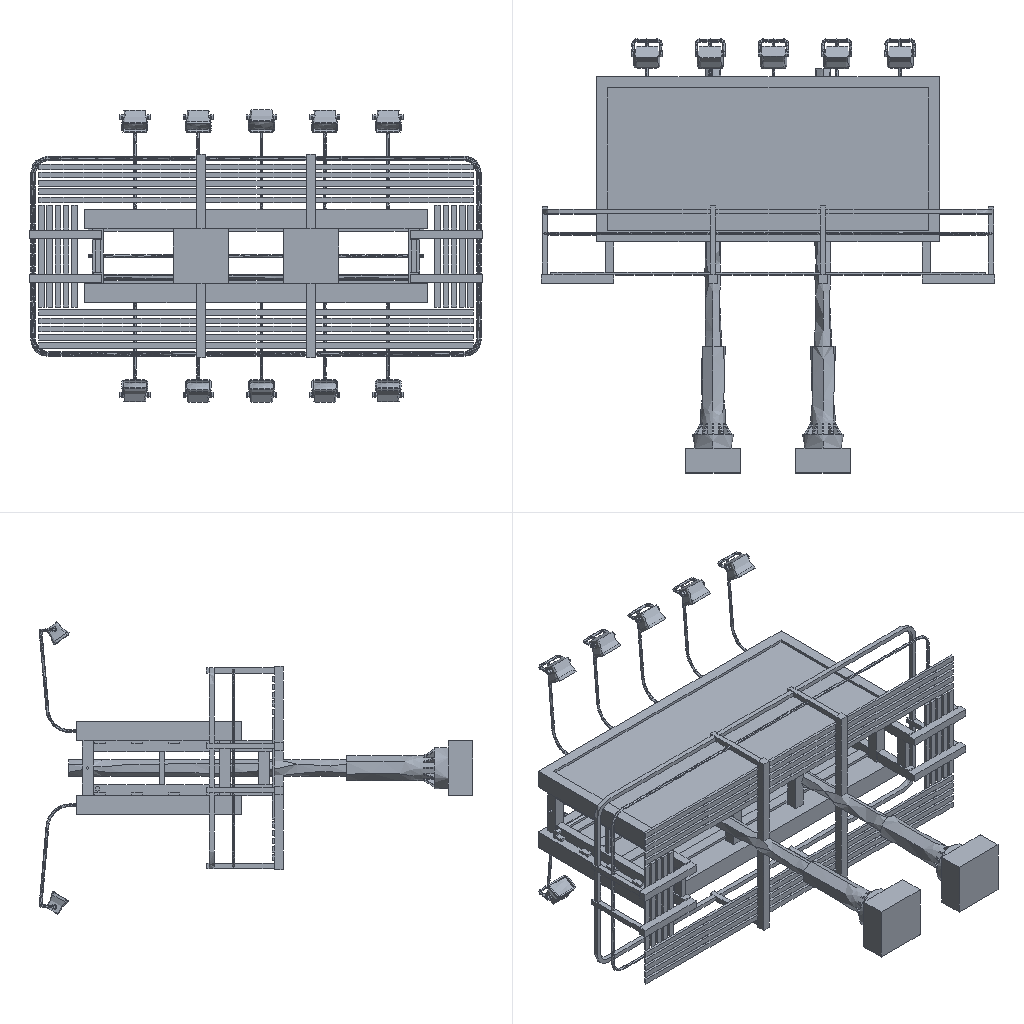Simulation study | ansys workbench
Set-up summary:
category,name,step,type,value,unit,region
solver,ansys_mapdl
solver,version,,,22.1
solver,version,,,22.1
units,MPA,,stated
analysis,deck1,,modal,modal
load_step,requested,,,1
analysis,nlgeom,,,False
mesh,nodes,,,79360
mesh,elements,,,41948
element_type,ANSYS 187 (type 1),,solid,28368
element_type,ANSYS 187 (type 2),,solid,916
element_type,ANSYS 187 (type 3),,solid,916
element_type,ANSYS 187 (type 4),,solid,916
element_type,ANSYS 187 (type 5),,solid,916
element_type,ANSYS 187 (type 6),,solid,916
element_type,ANSYS 187 (type 7),,solid,916
element_type,ANSYS 187 (type 8),,solid,916
element_type,ANSYS 187 (type 9),,solid,916
element_type,ANSYS 187 (type 10),,solid,916
element_type,ANSYS 187 (type 11),,solid,916
element_type,ANSYS 174 (type 12),,contact,216
element_type,ANSYS 170 (type 13),,target,216
element_type,ANSYS 174 (type 14),,contact,222
element_type,ANSYS 170 (type 15),,target,222
element_type,ANSYS 174 (type 16),,contact,214
element_type,ANSYS 170 (type 17),,target,214
element_type,ANSYS 174 (type 18),,contact,218
element_type,ANSYS 170 (type 19),,target,218
element_type,ANSYS 174 (type 20),,contact,221
element_type,ANSYS 170 (type 21),,target,221
element_type,ANSYS 174 (type 22),,contact,224
element_type,ANSYS 170 (type 23),,target,224
element_type,ANSYS 174 (type 24),,contact,226
element_type,ANSYS 170 (type 25),,target,226
element_type,ANSYS 174 (type 26),,contact,223
element_type,ANSYS 170 (type 27),,target,223
element_type,ANSYS 174 (type 28),,contact,220
element_type,ANSYS 170 (type 29),,target,220
element_type,ANSYS 174 (type 30),,contact,226
element_type,ANSYS 170 (type 31),,target,226
load,load commands in deck,,count,0
bc,support commands in deck,,count,0
analysis,deck2,,static,static
load_step,requested,,,1
analysis,nlgeom,,,False
mesh,nodes,,,79360
mesh,elements,,,42226
element_type,ANSYS 187 (type 1),,solid,28368
element_type,ANSYS 187 (type 2),,solid,916
element_type,ANSYS 187 (type 3),,solid,916
element_type,ANSYS 187 (type 4),,solid,916
element_type,ANSYS 187 (type 5),,solid,916
element_type,ANSYS 187 (type 6),,solid,916
element_type,ANSYS 187 (type 7),,solid,916
element_type,ANSYS 187 (type 8),,solid,916
element_type,ANSYS 187 (type 9),,solid,916
element_type,ANSYS 187 (type 10),,solid,916
element_type,ANSYS 187 (type 11),,solid,916
element_type,ANSYS 174 (type 12),,contact,216
element_type,ANSYS 170 (type 13),,target,216
element_type,ANSYS 174 (type 14),,contact,222
element_type,ANSYS 170 (type 15),,target,222
element_type,ANSYS 174 (type 16),,contact,214
element_type,ANSYS 170 (type 17),,target,214
element_type,ANSYS 174 (type 18),,contact,218
element_type,ANSYS 170 (type 19),,target,218
element_type,ANSYS 174 (type 20),,contact,221
element_type,ANSYS 170 (type 21),,target,221
element_type,ANSYS 174 (type 22),,contact,224
element_type,ANSYS 170 (type 23),,target,224
element_type,ANSYS 174 (type 24),,contact,226
element_type,ANSYS 170 (type 25),,target,226
element_type,ANSYS 174 (type 26),,contact,223
element_type,ANSYS 170 (type 27),,target,223
element_type,ANSYS 174 (type 28),,contact,220
element_type,ANSYS 170 (type 29),,target,220
element_type,ANSYS 174 (type 30),,contact,226
element_type,ANSYS 170 (type 31),,target,226
element_type,ANSYS 154 (type 32),,surface,278
load,load commands in deck,,count,3
bc,support commands in deck,,count,1
named_set,_FIXEDSU,,component
material,1,,in results
material,2,,in results
material,3,,in results
material,4,,in results
material,5,,in results
material,6,,in results
material,7,,in results
material,8,,in results
material,9,,in results
material,10,,in results
material,11,,in results
material,1,,in results
material,2,,in results
material,3,,in results
material,4,,in results
material,5,,in results
material,6,,in results
material,7,,in results
material,8,,in results
material,9,,in results
material,10,,in results
material,11,,in results
check,setup vs results,,match
check,setup vs results,,match,278 surface effect element(s) are not in the reader's mesh and were not compared
Results summary:
result,analysis,,,modal
result,last_loadstep,,,1
result,primary field,,,displacement
result,analysis,,,static
result,last_loadstep,,,1
result,primary field,,,displacement
result,reaction total,1,FX,8e-06,N
result,reaction total,1,FY,-1e-05,N
result,reaction total,1,FZ,5000,N
result,mass,,,1.043,"NMM: mm, ton, N, s, mV, mA, degC"